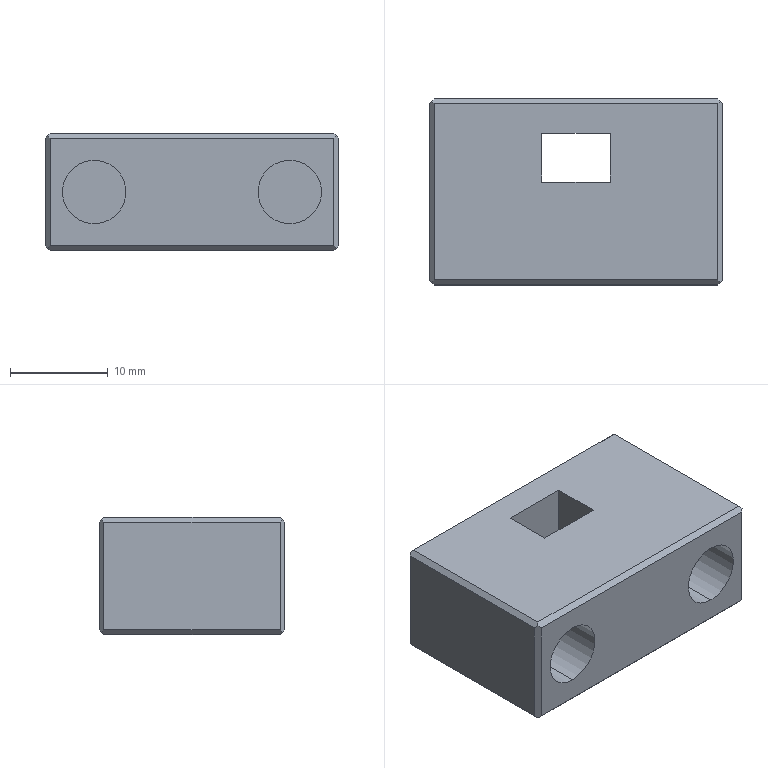Part | SolidWorks | features Chamfer 3, Cut 2, HoleWzd 2, Extrusion 1 | 1 solid | 52 faces | box 30 x 19 x 12 mm | volume 5175 mm3 | plane 24 | cone 16 | cylinder 12 | commonest cylinder face diameters 1.6 x4 3 x4 6.5 x4
STEP:
#1=CARTESIAN_POINT('',(12.5,9.3,-3.6));
#2=VERTEX_POINT('',#1);
#3=CARTESIAN_POINT('',(12.5,9.3,-2.));
#4=VERTEX_POINT('',#3);
#5=CARTESIAN_POINT('',(12.5,9.3,-2.8));
#6=DIRECTION('',(0.,1.,0.));
#7=DIRECTION('',(0.,0.,1.));
#8=AXIS2_PLACEMENT_3D('',#5,#6,#7);
#9=CIRCLE('',#8,0.8);
#10=EDGE_CURVE('',#2,#4,#9,.T.);
#11=ORIENTED_EDGE('',*,*,#10,.F.);
#12=CARTESIAN_POINT('',(12.5,9.5,-3.8));
#13=VERTEX_POINT('',#12);
#14=CARTESIAN_POINT('',(12.5,9.3,-3.6));
#15=DIRECTION('',(0.,0.7071,-0.7071));
#16=VECTOR('',#15,1000.);
#17=LINE('',#14,#16);
#18=EDGE_CURVE('',#2,#13,#17,.T.);
#19=ORIENTED_EDGE('',*,*,#18,.T.);
#20=CARTESIAN_POINT('',(12.5,9.5,-1.8));
#21=VERTEX_POINT('',#20);
#22=CARTESIAN_POINT('',(12.5,9.5,-2.8));
#23=DIRECTION('',(0.,-1.,0.));
#24=DIRECTION('',(0.,0.,1.));
#25=AXIS2_PLACEMENT_3D('',#22,#23,#24);
#26=CIRCLE('',#25,1.);
#27=EDGE_CURVE('',#21,#13,#26,.T.);
#28=ORIENTED_EDGE('',*,*,#27,.F.);
#29=CARTESIAN_POINT('',(12.5,9.3,-2.));
#30=DIRECTION('',(0.,0.7071,0.7071));
#31=VECTOR('',#30,1000.);
#32=LINE('',#29,#31);
#33=EDGE_CURVE('',#4,#21,#32,.T.);
#34=ORIENTED_EDGE('',*,*,#33,.F.);
#35=EDGE_LOOP('',(#11,#19,#28,#34));
#36=FACE_OUTER_BOUND('',#35,.T.);
#37=CARTESIAN_POINT('',(12.5,9.3,-2.8));
#38=DIRECTION('',(0.,1.,0.));
#39=DIRECTION('',(0.,0.,1.));
#40=AXIS2_PLACEMENT_3D('',#37,#38,#39);
#41=CONICAL_SURFACE('',#40,0.8,0.7854);
#42=ADVANCED_FACE('',(#36),#41,.F.);
#43=CARTESIAN_POINT('',(-12.5,9.3,-3.6));
#44=VERTEX_POINT('',#43);
#45=CARTESIAN_POINT('',(-12.5,9.3,-2.));
#46=VERTEX_POINT('',#45);
#47=CARTESIAN_POINT('',(-12.5,9.3,-2.8));
#48=DIRECTION('',(0.,1.,0.));
#49=DIRECTION('',(0.,0.,1.));
#50=AXIS2_PLACEMENT_3D('',#47,#48,#49);
#51=CIRCLE('',#50,0.8);
#52=EDGE_CURVE('',#44,#46,#51,.T.);
#53=ORIENTED_EDGE('',*,*,#52,.F.);
#54=CARTESIAN_POINT('',(-12.5,9.5,-3.8));
#55=VERTEX_POINT('',#54);
#56=CARTESIAN_POINT('',(-12.5,9.3,-3.6));
#57=DIRECTION('',(0.,0.7071,-0.7071));
#58=VECTOR('',#57,1000.);
#59=LINE('',#56,#58);
#60=EDGE_CURVE('',#44,#55,#59,.T.);
#61=ORIENTED_EDGE('',*,*,#60,.T.);
#62=CARTESIAN_POINT('',(-12.5,9.5,-1.8));
#63=VERTEX_POINT('',#62);
#64=CARTESIAN_POINT('',(-12.5,9.5,-2.8));
#65=DIRECTION('',(0.,-1.,0.));
#66=DIRECTION('',(0.,0.,1.));
#67=AXIS2_PLACEMENT_3D('',#64,#65,#66);
#68=CIRCLE('',#67,1.);
#69=EDGE_CURVE('',#63,#55,#68,.T.);
#70=ORIENTED_EDGE('',*,*,#69,.F.);
#71=CARTESIAN_POINT('',(-12.5,9.3,-2.));
#72=DIRECTION('',(0.,0.7071,0.7071));
#73=VECTOR('',#72,1000.);
#74=LINE('',#71,#73);
#75=EDGE_CURVE('',#46,#63,#74,.T.);
#76=ORIENTED_EDGE('',*,*,#75,.F.);
#77=EDGE_LOOP('',(#53,#61,#70,#76));
#78=FACE_OUTER_BOUND('',#77,.T.);
#79=CARTESIAN_POINT('',(-12.5,9.3,-2.8));
#80=DIRECTION('',(0.,1.,0.));
#81=DIRECTION('',(0.,0.,1.));
#82=AXIS2_PLACEMENT_3D('',#79,#80,#81);
#83=CONICAL_SURFACE('',#82,0.8,0.7854);
#84=ADVANCED_FACE('',(#78),#83,.F.);
#85=CARTESIAN_POINT('',(-6.,9.,-4.3));
#86=VERTEX_POINT('',#85);
#87=CARTESIAN_POINT('',(-6.,9.,-1.3));
#88=VERTEX_POINT('',#87);
#89=CARTESIAN_POINT('',(-6.,9.,-2.8));
#90=DIRECTION('',(0.,1.,0.));
#91=DIRECTION('',(0.,0.,1.));
#92=AXIS2_PLACEMENT_3D('',#89,#90,#91);
#93=CIRCLE('',#92,1.5);
#94=EDGE_CURVE('',#86,#88,#93,.T.);
#95=ORIENTED_EDGE('',*,*,#94,.F.);
#96=CARTESIAN_POINT('',(-6.,9.5,-4.8));
#97=VERTEX_POINT('',#96);
#98=CARTESIAN_POINT('',(-6.,9.,-4.3));
#99=DIRECTION('',(0.,0.7071,-0.7071));
#100=VECTOR('',#99,1000.);
#101=LINE('',#98,#100);
#102=EDGE_CURVE('',#86,#97,#101,.T.);
#103=ORIENTED_EDGE('',*,*,#102,.T.);
#104=CARTESIAN_POINT('',(-6.,9.5,-0.8));
#105=VERTEX_POINT('',#104);
#106=CARTESIAN_POINT('',(-6.,9.5,-2.8));
#107=DIRECTION('',(0.,-1.,0.));
#108=DIRECTION('',(0.,0.,1.));
#109=AXIS2_PLACEMENT_3D('',#106,#107,#108);
#110=CIRCLE('',#109,2.);
#111=EDGE_CURVE('',#105,#97,#110,.T.);
#112=ORIENTED_EDGE('',*,*,#111,.F.);
#113=CARTESIAN_POINT('',(-6.,9.,-1.3));
#114=DIRECTION('',(0.,0.7071,0.7071));
#115=VECTOR('',#114,1000.);
#116=LINE('',#113,#115);
#117=EDGE_CURVE('',#88,#105,#116,.T.);
#118=ORIENTED_EDGE('',*,*,#117,.F.);
#119=EDGE_LOOP('',(#95,#103,#112,#118));
#120=FACE_OUTER_BOUND('',#119,.T.);
#121=CARTESIAN_POINT('',(-6.,9.,-2.8));
#122=DIRECTION('',(0.,1.,0.));
#123=DIRECTION('',(0.,0.,1.));
#124=AXIS2_PLACEMENT_3D('',#121,#122,#123);
#125=CONICAL_SURFACE('',#124,1.5,0.7854);
#126=ADVANCED_FACE('',(#120),#125,.F.);
#127=CARTESIAN_POINT('',(6.,9.,-4.3));
#128=VERTEX_POINT('',#127);
#129=CARTESIAN_POINT('',(6.,9.,-1.3));
#130=VERTEX_POINT('',#129);
#131=CARTESIAN_POINT('',(6.,9.,-2.8));
#132=DIRECTION('',(0.,1.,0.));
#133=DIRECTION('',(0.,0.,1.));
#134=AXIS2_PLACEMENT_3D('',#131,#132,#133);
#135=CIRCLE('',#134,1.5);
#136=EDGE_CURVE('',#128,#130,#135,.T.);
#137=ORIENTED_EDGE('',*,*,#136,.F.);
#138=CARTESIAN_POINT('',(6.,9.5,-4.8));
#139=VERTEX_POINT('',#138);
#140=CARTESIAN_POINT('',(6.,9.,-4.3));
#141=DIRECTION('',(0.,0.7071,-0.7071));
#142=VECTOR('',#141,1000.);
#143=LINE('',#140,#142);
#144=EDGE_CURVE('',#128,#139,#143,.T.);
#145=ORIENTED_EDGE('',*,*,#144,.T.);
#146=CARTESIAN_POINT('',(6.,9.5,-0.8));
#147=VERTEX_POINT('',#146);
#148=CARTESIAN_POINT('',(6.,9.5,-2.8));
#149=DIRECTION('',(0.,-1.,0.));
#150=DIRECTION('',(0.,0.,1.));
#151=AXIS2_PLACEMENT_3D('',#148,#149,#150);
#152=CIRCLE('',#151,2.);
#153=EDGE_CURVE('',#147,#139,#152,.T.);
#154=ORIENTED_EDGE('',*,*,#153,.F.);
#155=CARTESIAN_POINT('',(6.,9.,-1.3));
#156=DIRECTION('',(0.,0.7071,0.7071));
#157=VECTOR('',#156,1000.);
#158=LINE('',#155,#157);
#159=EDGE_CURVE('',#130,#147,#158,.T.);
#160=ORIENTED_EDGE('',*,*,#159,.F.);
#161=EDGE_LOOP('',(#137,#145,#154,#160));
#162=FACE_OUTER_BOUND('',#161,.T.);
#163=CARTESIAN_POINT('',(6.,9.,-2.8));
#164=DIRECTION('',(0.,1.,0.));
#165=DIRECTION('',(0.,0.,1.));
#166=AXIS2_PLACEMENT_3D('',#163,#164,#165);
#167=CONICAL_SURFACE('',#166,1.5,0.7854);
#168=ADVANCED_FACE('',(#162),#167,.F.);
#169=CARTESIAN_POINT('',(6.,2.5,-4.3));
#170=VERTEX_POINT('',#169);
#171=CARTESIAN_POINT('',(6.,2.5,-1.3));
#172=VERTEX_POINT('',#171);
#173=CARTESIAN_POINT('',(6.,2.5,-2.8));
#174=DIRECTION('',(0.,1.,0.));
#175=DIRECTION('',(0.,0.,1.));
#176=AXIS2_PLACEMENT_3D('',#173,#174,#175);
#177=CIRCLE('',#176,1.5);
#178=EDGE_CURVE('',#170,#172,#177,.T.);
#179=ORIENTED_EDGE('',*,*,#178,.F.);
#180=CARTESIAN_POINT('',(6.,9.5,-4.3));
#181=DIRECTION('',(0.,1.,0.));
#182=VECTOR('',#181,1000.);
#183=LINE('',#180,#182);
#184=EDGE_CURVE('',#170,#128,#183,.T.);
#185=ORIENTED_EDGE('',*,*,#184,.T.);
#186=ORIENTED_EDGE('',*,*,#136,.T.);
#187=CARTESIAN_POINT('',(6.,9.5,-1.3));
#188=DIRECTION('',(0.,1.,0.));
#189=VECTOR('',#188,1000.);
#190=LINE('',#187,#189);
#191=EDGE_CURVE('',#172,#130,#190,.T.);
#192=ORIENTED_EDGE('',*,*,#191,.F.);
#193=EDGE_LOOP('',(#179,#185,#186,#192));
#194=FACE_OUTER_BOUND('',#193,.T.);
#195=CARTESIAN_POINT('',(6.,9.5,-2.8));
#196=DIRECTION('',(0.,1.,0.));
#197=DIRECTION('',(0.,0.,1.));
#198=AXIS2_PLACEMENT_3D('',#195,#196,#197);
#199=CYLINDRICAL_SURFACE('',#198,1.5);
#200=ADVANCED_FACE('',(#194),#199,.F.);
#201=CARTESIAN_POINT('',(6.,1.599,-2.8));
#202=VERTEX_POINT('',#201);
#203=CARTESIAN_POINT('',(6.,2.5,-1.3));
#204=DIRECTION('',(0.,0.515,0.8572));
#205=VECTOR('',#204,1000.);
#206=LINE('',#203,#205);
#207=EDGE_CURVE('',#202,#172,#206,.T.);
#208=ORIENTED_EDGE('',*,*,#207,.F.);
#209=CARTESIAN_POINT('',(6.,2.5,-4.3));
#210=DIRECTION('',(0.,0.515,-0.8572));
#211=VECTOR('',#210,1000.);
#212=LINE('',#209,#211);
#213=EDGE_CURVE('',#202,#170,#212,.T.);
#214=ORIENTED_EDGE('',*,*,#213,.T.);
#215=ORIENTED_EDGE('',*,*,#178,.T.);
#216=EDGE_LOOP('',(#208,#214,#215));
#217=FACE_OUTER_BOUND('',#216,.T.);
#218=CARTESIAN_POINT('',(6.,2.5,-2.8));
#219=DIRECTION('',(0.,1.,0.));
#220=DIRECTION('',(0.,0.,1.));
#221=AXIS2_PLACEMENT_3D('',#218,#219,#220);
#222=CONICAL_SURFACE('',#221,1.5,1.03);
#223=ADVANCED_FACE('',(#217),#222,.F.);
#224=CARTESIAN_POINT('',(-6.,2.5,-4.3));
#225=VERTEX_POINT('',#224);
#226=CARTESIAN_POINT('',(-6.,2.5,-1.3));
#227=VERTEX_POINT('',#226);
#228=CARTESIAN_POINT('',(-6.,2.5,-2.8));
#229=DIRECTION('',(0.,1.,0.));
#230=DIRECTION('',(0.,0.,1.));
#231=AXIS2_PLACEMENT_3D('',#228,#229,#230);
#232=CIRCLE('',#231,1.5);
#233=EDGE_CURVE('',#225,#227,#232,.T.);
#234=ORIENTED_EDGE('',*,*,#233,.F.);
#235=CARTESIAN_POINT('',(-6.,9.5,-4.3));
#236=DIRECTION('',(0.,1.,0.));
#237=VECTOR('',#236,1000.);
#238=LINE('',#235,#237);
#239=EDGE_CURVE('',#225,#86,#238,.T.);
#240=ORIENTED_EDGE('',*,*,#239,.T.);
#241=ORIENTED_EDGE('',*,*,#94,.T.);
#242=CARTESIAN_POINT('',(-6.,9.5,-1.3));
#243=DIRECTION('',(0.,1.,0.));
#244=VECTOR('',#243,1000.);
#245=LINE('',#242,#244);
#246=EDGE_CURVE('',#227,#88,#245,.T.);
#247=ORIENTED_EDGE('',*,*,#246,.F.);
#248=EDGE_LOOP('',(#234,#240,#241,#247));
#249=FACE_OUTER_BOUND('',#248,.T.);
#250=CARTESIAN_POINT('',(-6.,9.5,-2.8));
#251=DIRECTION('',(0.,1.,0.));
#252=DIRECTION('',(0.,0.,1.));
#253=AXIS2_PLACEMENT_3D('',#250,#251,#252);
#254=CYLINDRICAL_SURFACE('',#253,1.5);
#255=ADVANCED_FACE('',(#249),#254,.F.);
#256=CARTESIAN_POINT('',(-6.,1.599,-2.8));
#257=VERTEX_POINT('',#256);
#258=CARTESIAN_POINT('',(-6.,2.5,-1.3));
#259=DIRECTION('',(0.,0.515,0.8572));
#260=VECTOR('',#259,1000.);
#261=LINE('',#258,#260);
#262=EDGE_CURVE('',#257,#227,#261,.T.);
#263=ORIENTED_EDGE('',*,*,#262,.F.);
#264=CARTESIAN_POINT('',(-6.,2.5,-4.3));
#265=DIRECTION('',(0.,0.515,-0.8572));
#266=VECTOR('',#265,1000.);
#267=LINE('',#264,#266);
#268=EDGE_CURVE('',#257,#225,#267,.T.);
#269=ORIENTED_EDGE('',*,*,#268,.T.);
#270=ORIENTED_EDGE('',*,*,#233,.T.);
#271=EDGE_LOOP('',(#263,#269,#270));
#272=FACE_OUTER_BOUND('',#271,.T.);
#273=CARTESIAN_POINT('',(-6.,2.5,-2.8));
#274=DIRECTION('',(0.,1.,0.));
#275=DIRECTION('',(0.,0.,1.));
#276=AXIS2_PLACEMENT_3D('',#273,#274,#275);
#277=CONICAL_SURFACE('',#276,1.5,1.03);
#278=ADVANCED_FACE('',(#272),#277,.F.);
#279=CARTESIAN_POINT('',(-12.5,4.3,-3.6));
#280=VERTEX_POINT('',#279);
#281=CARTESIAN_POINT('',(-12.5,4.3,-2.));
#282=VERTEX_POINT('',#281);
#283=CARTESIAN_POINT('',(-12.5,4.3,-2.8));
#284=DIRECTION('',(0.,1.,0.));
#285=DIRECTION('',(0.,0.,1.));
#286=AXIS2_PLACEMENT_3D('',#283,#284,#285);
#287=CIRCLE('',#286,0.8);
#288=EDGE_CURVE('',#280,#282,#287,.T.);
#289=ORIENTED_EDGE('',*,*,#288,.F.);
#290=CARTESIAN_POINT('',(-12.5,9.5,-3.6));
#291=DIRECTION('',(0.,1.,0.));
#292=VECTOR('',#291,1000.);
#293=LINE('',#290,#292);
#294=EDGE_CURVE('',#280,#44,#293,.T.);
#295=ORIENTED_EDGE('',*,*,#294,.T.);
#296=ORIENTED_EDGE('',*,*,#52,.T.);
#297=CARTESIAN_POINT('',(-12.5,9.5,-2.));
#298=DIRECTION('',(0.,1.,0.));
#299=VECTOR('',#298,1000.);
#300=LINE('',#297,#299);
#301=EDGE_CURVE('',#282,#46,#300,.T.);
#302=ORIENTED_EDGE('',*,*,#301,.F.);
#303=EDGE_LOOP('',(#289,#295,#296,#302));
#304=FACE_OUTER_BOUND('',#303,.T.);
#305=CARTESIAN_POINT('',(-12.5,9.5,-2.8));
#306=DIRECTION('',(0.,1.,0.));
#307=DIRECTION('',(0.,0.,1.));
#308=AXIS2_PLACEMENT_3D('',#305,#306,#307);
#309=CYLINDRICAL_SURFACE('',#308,0.8);
#310=ADVANCED_FACE('',(#304),#309,.F.);
#311=CARTESIAN_POINT('',(-12.5,3.819,-2.8));
#312=VERTEX_POINT('',#311);
#313=CARTESIAN_POINT('',(-12.5,4.3,-2.));
#314=DIRECTION('',(0.,0.515,0.8572));
#315=VECTOR('',#314,1000.);
#316=LINE('',#313,#315);
#317=EDGE_CURVE('',#312,#282,#316,.T.);
#318=ORIENTED_EDGE('',*,*,#317,.F.);
#319=CARTESIAN_POINT('',(-12.5,4.3,-3.6));
#320=DIRECTION('',(0.,0.515,-0.8572));
#321=VECTOR('',#320,1000.);
#322=LINE('',#319,#321);
#323=EDGE_CURVE('',#312,#280,#322,.T.);
#324=ORIENTED_EDGE('',*,*,#323,.T.);
#325=ORIENTED_EDGE('',*,*,#288,.T.);
#326=EDGE_LOOP('',(#318,#324,#325));
#327=FACE_OUTER_BOUND('',#326,.T.);
#328=CARTESIAN_POINT('',(-12.5,4.3,-2.8));
#329=DIRECTION('',(0.,1.,0.));
#330=DIRECTION('',(0.,0.,1.));
#331=AXIS2_PLACEMENT_3D('',#328,#329,#330);
#332=CONICAL_SURFACE('',#331,0.8,1.03);
#333=ADVANCED_FACE('',(#327),#332,.F.);
#334=CARTESIAN_POINT('',(12.5,4.3,-3.6));
#335=VERTEX_POINT('',#334);
#336=CARTESIAN_POINT('',(12.5,4.3,-2.));
#337=VERTEX_POINT('',#336);
#338=CARTESIAN_POINT('',(12.5,4.3,-2.8));
#339=DIRECTION('',(0.,1.,0.));
#340=DIRECTION('',(0.,0.,1.));
#341=AXIS2_PLACEMENT_3D('',#338,#339,#340);
#342=CIRCLE('',#341,0.8);
#343=EDGE_CURVE('',#335,#337,#342,.T.);
#344=ORIENTED_EDGE('',*,*,#343,.F.);
#345=CARTESIAN_POINT('',(12.5,9.5,-3.6));
#346=DIRECTION('',(0.,1.,0.));
#347=VECTOR('',#346,1000.);
#348=LINE('',#345,#347);
#349=EDGE_CURVE('',#335,#2,#348,.T.);
#350=ORIENTED_EDGE('',*,*,#349,.T.);
#351=ORIENTED_EDGE('',*,*,#10,.T.);
#352=CARTESIAN_POINT('',(12.5,9.5,-2.));
#353=DIRECTION('',(0.,1.,0.));
#354=VECTOR('',#353,1000.);
#355=LINE('',#352,#354);
#356=EDGE_CURVE('',#337,#4,#355,.T.);
#357=ORIENTED_EDGE('',*,*,#356,.F.);
#358=EDGE_LOOP('',(#344,#350,#351,#357));
#359=FACE_OUTER_BOUND('',#358,.T.);
#360=CARTESIAN_POINT('',(12.5,9.5,-2.8));
#361=DIRECTION('',(0.,1.,0.));
#362=DIRECTION('',(0.,0.,1.));
#363=AXIS2_PLACEMENT_3D('',#360,#361,#362);
#364=CYLINDRICAL_SURFACE('',#363,0.8);
#365=ADVANCED_FACE('',(#359),#364,.F.);
#366=CARTESIAN_POINT('',(12.5,3.819,-2.8));
#367=VERTEX_POINT('',#366);
#368=CARTESIAN_POINT('',(12.5,4.3,-2.));
#369=DIRECTION('',(0.,0.515,0.8572));
#370=VECTOR('',#369,1000.);
#371=LINE('',#368,#370);
#372=EDGE_CURVE('',#367,#337,#371,.T.);
#373=ORIENTED_EDGE('',*,*,#372,.F.);
#374=CARTESIAN_POINT('',(12.5,4.3,-3.6));
#375=DIRECTION('',(0.,0.515,-0.8572));
#376=VECTOR('',#375,1000.);
#377=LINE('',#374,#376);
#378=EDGE_CURVE('',#367,#335,#377,.T.);
#379=ORIENTED_EDGE('',*,*,#378,.T.);
#380=ORIENTED_EDGE('',*,*,#343,.T.);
#381=EDGE_LOOP('',(#373,#379,#380));
#382=FACE_OUTER_BOUND('',#381,.T.);
#383=CARTESIAN_POINT('',(12.5,4.3,-2.8));
#384=DIRECTION('',(0.,1.,0.));
#385=DIRECTION('',(0.,0.,1.));
#386=AXIS2_PLACEMENT_3D('',#383,#384,#385);
#387=CONICAL_SURFACE('',#386,0.8,1.03);
#388=ADVANCED_FACE('',(#382),#387,.F.);
#389=CARTESIAN_POINT('',(-10.,2.5,-9.25));
#390=VERTEX_POINT('',#389);
#391=CARTESIAN_POINT('',(-10.,2.5,-2.75));
#392=VERTEX_POINT('',#391);
#393=CARTESIAN_POINT('',(-10.,2.5,-6.));
#394=DIRECTION('',(0.,1.,0.));
#395=DIRECTION('',(0.,0.,-1.));
#396=AXIS2_PLACEMENT_3D('',#393,#394,#395);
#397=CIRCLE('',#396,3.25);
#398=EDGE_CURVE('',#390,#392,#397,.T.);
#399=ORIENTED_EDGE('',*,*,#398,.T.);
#400=CARTESIAN_POINT('',(-10.,-9.5,-2.75));
#401=VERTEX_POINT('',#400);
#402=CARTESIAN_POINT('',(-10.,11.692,-2.75));
#403=DIRECTION('',(0.,-1.,0.));
#404=VECTOR('',#403,1000.);
#405=LINE('',#402,#404);
#406=EDGE_CURVE('',#392,#401,#405,.T.);
#407=ORIENTED_EDGE('',*,*,#406,.T.);
#408=CARTESIAN_POINT('',(-10.,-9.5,-9.25));
#409=VERTEX_POINT('',#408);
#410=CARTESIAN_POINT('',(-10.,-9.5,-6.));
#411=DIRECTION('',(0.,-1.,0.));
#412=DIRECTION('',(0.,0.,-1.));
#413=AXIS2_PLACEMENT_3D('',#410,#411,#412);
#414=CIRCLE('',#413,3.25);
#415=EDGE_CURVE('',#401,#409,#414,.T.);
#416=ORIENTED_EDGE('',*,*,#415,.T.);
#417=CARTESIAN_POINT('',(-10.,11.692,-9.25));
#418=DIRECTION('',(0.,-1.,0.));
#419=VECTOR('',#418,1000.);
#420=LINE('',#417,#419);
#421=EDGE_CURVE('',#390,#409,#420,.T.);
#422=ORIENTED_EDGE('',*,*,#421,.F.);
#423=EDGE_LOOP('',(#399,#407,#416,#422));
#424=FACE_OUTER_BOUND('',#423,.T.);
#425=CARTESIAN_POINT('',(-10.,11.692,-6.));
#426=DIRECTION('',(0.,-1.,0.));
#427=DIRECTION('',(0.,0.,-1.));
#428=AXIS2_PLACEMENT_3D('',#425,#426,#427);
#429=CYLINDRICAL_SURFACE('',#428,3.25);
#430=ADVANCED_FACE('',(#424),#429,.F.);
#431=CARTESIAN_POINT('',(10.,2.5,-2.75));
#432=VERTEX_POINT('',#431);
#433=CARTESIAN_POINT('',(10.,2.5,-9.25));
#434=VERTEX_POINT('',#433);
#435=CARTESIAN_POINT('',(10.,2.5,-6.));
#436=DIRECTION('',(0.,-1.,0.));
#437=DIRECTION('',(0.,0.,-1.));
#438=AXIS2_PLACEMENT_3D('',#435,#436,#437);
#439=CIRCLE('',#438,3.25);
#440=EDGE_CURVE('',#432,#434,#439,.T.);
#441=ORIENTED_EDGE('',*,*,#440,.F.);
#442=CARTESIAN_POINT('',(10.,-9.5,-2.75));
#443=VERTEX_POINT('',#442);
#444=CARTESIAN_POINT('',(10.,11.692,-2.75));
#445=DIRECTION('',(0.,-1.,0.));
#446=VECTOR('',#445,1000.);
#447=LINE('',#444,#446);
#448=EDGE_CURVE('',#432,#443,#447,.T.);
#449=ORIENTED_EDGE('',*,*,#448,.T.);
#450=CARTESIAN_POINT('',(10.,-9.5,-9.25));
#451=VERTEX_POINT('',#450);
#452=CARTESIAN_POINT('',(10.,-9.5,-6.));
#453=DIRECTION('',(0.,-1.,0.));
#454=DIRECTION('',(0.,0.,-1.));
#455=AXIS2_PLACEMENT_3D('',#452,#453,#454);
#456=CIRCLE('',#455,3.25);
#457=EDGE_CURVE('',#443,#451,#456,.T.);
#458=ORIENTED_EDGE('',*,*,#457,.T.);
#459=CARTESIAN_POINT('',(10.,11.692,-9.25));
#460=DIRECTION('',(0.,-1.,0.));
#461=VECTOR('',#460,1000.);
#462=LINE('',#459,#461);
#463=EDGE_CURVE('',#434,#451,#462,.T.);
#464=ORIENTED_EDGE('',*,*,#463,.F.);
#465=EDGE_LOOP('',(#441,#449,#458,#464));
#466=FACE_OUTER_BOUND('',#465,.T.);
#467=CARTESIAN_POINT('',(10.,11.692,-6.));
#468=DIRECTION('',(0.,-1.,0.));
#469=DIRECTION('',(0.,0.,-1.));
#470=AXIS2_PLACEMENT_3D('',#467,#468,#469);
#471=CYLINDRICAL_SURFACE('',#470,3.25);
#472=ADVANCED_FACE('',(#466),#471,.F.);
#473=CARTESIAN_POINT('',(14.5,-9.,0.));
#474=VERTEX_POINT('',#473);
#475=CARTESIAN_POINT('',(14.5,9.,0.));
#476=VERTEX_POINT('',#475);
#477=CARTESIAN_POINT('',(14.5,0.,0.));
#478=DIRECTION('',(0.,1.,0.));
#479=VECTOR('',#478,1000.);
#480=LINE('',#477,#479);
#481=EDGE_CURVE('',#474,#476,#480,.T.);
#482=ORIENTED_EDGE('',*,*,#481,.T.);
#483=CARTESIAN_POINT('',(-14.5,9.,0.));
#484=VERTEX_POINT('',#483);
#485=CARTESIAN_POINT('',(0.,9.,0.));
#486=DIRECTION('',(-1.,0.,0.));
#487=VECTOR('',#486,1000.);
#488=LINE('',#485,#487);
#489=EDGE_CURVE('',#476,#484,#488,.T.);
#490=ORIENTED_EDGE('',*,*,#489,.T.);
#491=CARTESIAN_POINT('',(-14.5,-9.,0.));
#492=VERTEX_POINT('',#491);
#493=CARTESIAN_POINT('',(-14.5,0.,0.));
#494=DIRECTION('',(0.,-1.,0.));
#495=VECTOR('',#494,1000.);
#496=LINE('',#493,#495);
#497=EDGE_CURVE('',#484,#492,#496,.T.);
#498=ORIENTED_EDGE('',*,*,#497,.T.);
#499=CARTESIAN_POINT('',(0.,-9.,0.));
#500=DIRECTION('',(1.,0.,0.));
#501=VECTOR('',#500,1000.);
#502=LINE('',#499,#501);
#503=EDGE_CURVE('',#492,#474,#502,.T.);
#504=ORIENTED_EDGE('',*,*,#503,.T.);
#505=EDGE_LOOP('',(#482,#490,#498,#504));
#506=FACE_OUTER_BOUND('',#505,.T.);
#507=CARTESIAN_POINT('',(3.5,1.,0.));
#508=VERTEX_POINT('',#507);
#509=CARTESIAN_POINT('',(-3.5,1.,0.));
#510=VERTEX_POINT('',#509);
#511=CARTESIAN_POINT('',(20.42,1.,0.));
#512=DIRECTION('',(-1.,0.,0.));
#513=VECTOR('',#512,1000.);
#514=LINE('',#511,#513);
#515=EDGE_CURVE('',#508,#510,#514,.T.);
#516=ORIENTED_EDGE('',*,*,#515,.T.);
#517=CARTESIAN_POINT('',(-3.5,6.,0.));
#518=VERTEX_POINT('',#517);
#519=CARTESIAN_POINT('',(-3.5,6.,0.));
#520=DIRECTION('',(0.,-1.,0.));
#521=VECTOR('',#520,1000.);
#522=LINE('',#519,#521);
#523=EDGE_CURVE('',#518,#510,#522,.T.);
#524=ORIENTED_EDGE('',*,*,#523,.F.);
#525=CARTESIAN_POINT('',(3.5,6.,0.));
#526=VERTEX_POINT('',#525);
#527=CARTESIAN_POINT('',(20.42,6.,0.));
#528=DIRECTION('',(-1.,0.,0.));
#529=VECTOR('',#528,1000.);
#530=LINE('',#527,#529);
#531=EDGE_CURVE('',#526,#518,#530,.T.);
#532=ORIENTED_EDGE('',*,*,#531,.F.);
#533=CARTESIAN_POINT('',(3.5,6.,0.));
#534=DIRECTION('',(0.,-1.,0.));
#535=VECTOR('',#534,1000.);
#536=LINE('',#533,#535);
#537=EDGE_CURVE('',#526,#508,#536,.T.);
#538=ORIENTED_EDGE('',*,*,#537,.T.);
#539=EDGE_LOOP('',(#516,#524,#532,#538));
#540=FACE_BOUND('',#539,.T.);
#541=CARTESIAN_POINT('',(0.,0.,0.));
#542=DIRECTION('',(0.,0.,1.));
#543=DIRECTION('',(1.,0.,0.));
#544=AXIS2_PLACEMENT_3D('',#541,#542,#543);
#545=PLANE('',#544);
#546=ADVANCED_FACE('',(#506,#540),#545,.T.);
#547=CARTESIAN_POINT('',(-14.5,9.,-12.));
#548=VERTEX_POINT('',#547);
#549=CARTESIAN_POINT('',(14.5,9.,-12.));
#550=VERTEX_POINT('',#549);
#551=CARTESIAN_POINT('',(14.5,9.,-12.));
#552=DIRECTION('',(1.,0.,0.));
#553=VECTOR('',#552,1000.);
#554=LINE('',#551,#553);
#555=EDGE_CURVE('',#548,#550,#554,.T.);
#556=ORIENTED_EDGE('',*,*,#555,.T.);
#557=CARTESIAN_POINT('',(14.5,-9.,-12.));
#558=VERTEX_POINT('',#557);
#559=CARTESIAN_POINT('',(14.5,-9.,-12.));
#560=DIRECTION('',(0.,-1.,0.));
#561=VECTOR('',#560,1000.);
#562=LINE('',#559,#561);
#563=EDGE_CURVE('',#550,#558,#562,.T.);
#564=ORIENTED_EDGE('',*,*,#563,.T.);
#565=CARTESIAN_POINT('',(-14.5,-9.,-12.));
#566=VERTEX_POINT('',#565);
#567=CARTESIAN_POINT('',(-14.5,-9.,-12.));
#568=DIRECTION('',(-1.,0.,0.));
#569=VECTOR('',#568,1000.);
#570=LINE('',#567,#569);
#571=EDGE_CURVE('',#558,#566,#570,.T.);
#572=ORIENTED_EDGE('',*,*,#571,.T.);
#573=CARTESIAN_POINT('',(-14.5,9.,-12.));
#574=DIRECTION('',(0.,1.,0.));
#575=VECTOR('',#574,1000.);
#576=LINE('',#573,#575);
#577=EDGE_CURVE('',#566,#548,#576,.T.);
#578=ORIENTED_EDGE('',*,*,#577,.T.);
#579=EDGE_LOOP('',(#556,#564,#572,#578));
#580=FACE_OUTER_BOUND('',#579,.T.);
#581=CARTESIAN_POINT('',(-3.5,-5.928,-12.));
#582=VERTEX_POINT('',#581);
#583=CARTESIAN_POINT('',(-3.5,6.,-12.));
#584=VERTEX_POINT('',#583);
#585=CARTESIAN_POINT('',(-3.5,-5.928,-12.));
#586=DIRECTION('',(0.,1.,0.));
#587=VECTOR('',#586,1000.);
#588=LINE('',#585,#587);
#589=EDGE_CURVE('',#582,#584,#588,.T.);
#590=ORIENTED_EDGE('',*,*,#589,.F.);
#591=CARTESIAN_POINT('',(3.5,-5.928,-12.));
#592=VERTEX_POINT('',#591);
#593=CARTESIAN_POINT('',(20.42,-5.928,-12.));
#594=DIRECTION('',(-1.,0.,0.));
#595=VECTOR('',#594,1000.);
#596=LINE('',#593,#595);
#597=EDGE_CURVE('',#592,#582,#596,.T.);
#598=ORIENTED_EDGE('',*,*,#597,.F.);
#599=CARTESIAN_POINT('',(3.5,6.,-12.));
#600=VERTEX_POINT('',#599);
#601=CARTESIAN_POINT('',(3.5,-5.928,-12.));
#602=DIRECTION('',(0.,1.,0.));
#603=VECTOR('',#602,1000.);
#604=LINE('',#601,#603);
#605=EDGE_CURVE('',#592,#600,#604,.T.);
#606=ORIENTED_EDGE('',*,*,#605,.T.);
#607=CARTESIAN_POINT('',(20.42,6.,-12.));
#608=DIRECTION('',(-1.,0.,0.));
#609=VECTOR('',#608,1000.);
#610=LINE('',#607,#609);
#611=EDGE_CURVE('',#600,#584,#610,.T.);
#612=ORIENTED_EDGE('',*,*,#611,.T.);
#613=EDGE_LOOP('',(#590,#598,#606,#612));
#614=FACE_BOUND('',#613,.T.);
#615=CARTESIAN_POINT('',(0.,0.,-12.));
#616=DIRECTION('',(0.,0.,1.));
#617=DIRECTION('',(1.,0.,0.));
#618=AXIS2_PLACEMENT_3D('',#615,#616,#617);
#619=PLANE('',#618);
#620=ADVANCED_FACE('',(#580,#614),#619,.F.);
#621=CARTESIAN_POINT('',(-14.5,9.5,-11.5));
#622=VERTEX_POINT('',#621);
#623=CARTESIAN_POINT('',(-14.5,9.5,-0.5));
#624=VERTEX_POINT('',#623);
#625=CARTESIAN_POINT('',(-14.5,9.5,-47.511));
#626=DIRECTION('',(0.,0.,1.));
#627=VECTOR('',#626,1000.);
#628=LINE('',#625,#627);
#629=EDGE_CURVE('',#622,#624,#628,.T.);
#630=ORIENTED_EDGE('',*,*,#629,.F.);
#631=CARTESIAN_POINT('',(-14.75,9.25,-11.75));
#632=VERTEX_POINT('',#631);
#633=CARTESIAN_POINT('',(-26.504,-2.504,-23.504));
#634=DIRECTION('',(-0.5774,-0.5774,-0.5774));
#635=VECTOR('',#634,1000.);
#636=LINE('',#633,#635);
#637=EDGE_CURVE('',#622,#632,#636,.T.);
#638=ORIENTED_EDGE('',*,*,#637,.T.);
#639=CARTESIAN_POINT('',(-15.,9.,-11.5));
#640=VERTEX_POINT('',#639);
#641=CARTESIAN_POINT('',(-2.663,21.337,-23.837));
#642=DIRECTION('',(-0.5774,-0.5774,0.5774));
#643=VECTOR('',#642,1000.);
#644=LINE('',#641,#643);
#645=EDGE_CURVE('',#632,#640,#644,.T.);
#646=ORIENTED_EDGE('',*,*,#645,.T.);
#647=CARTESIAN_POINT('',(-15.,9.,-0.5));
#648=VERTEX_POINT('',#647);
#649=CARTESIAN_POINT('',(-15.,9.,-47.511));
#650=DIRECTION('',(0.,0.,1.));
#651=VECTOR('',#650,1000.);
#652=LINE('',#649,#651);
#653=EDGE_CURVE('',#640,#648,#652,.T.);
#654=ORIENTED_EDGE('',*,*,#653,.T.);
#655=CARTESIAN_POINT('',(-14.75,9.25,-0.25));
#656=VERTEX_POINT('',#655);
#657=CARTESIAN_POINT('',(-30.337,-6.337,-15.837));
#658=DIRECTION('',(0.5774,0.5774,0.5774));
#659=VECTOR('',#658,1000.);
#660=LINE('',#657,#659);
#661=EDGE_CURVE('',#648,#656,#660,.T.);
#662=ORIENTED_EDGE('',*,*,#661,.T.);
#663=CARTESIAN_POINT('',(1.17,25.17,-16.17));
#664=DIRECTION('',(0.5774,0.5774,-0.5774));
#665=VECTOR('',#664,1000.);
#666=LINE('',#663,#665);
#667=EDGE_CURVE('',#656,#624,#666,.T.);
#668=ORIENTED_EDGE('',*,*,#667,.T.);
#669=EDGE_LOOP('',(#630,#638,#646,#654,#662,#668));
#670=FACE_OUTER_BOUND('',#669,.T.);
#671=CARTESIAN_POINT('',(-14.5,9.5,-47.511));
#672=DIRECTION('',(-0.7071,0.7071,0.));
#673=DIRECTION('',(-0.7071,-0.7071,0.));
#674=AXIS2_PLACEMENT_3D('',#671,#672,#673);
#675=PLANE('',#674);
#676=ADVANCED_FACE('',(#670),#675,.T.);
#677=ORIENTED_EDGE('',*,*,#69,.T.);
#678=CARTESIAN_POINT('',(-12.5,9.5,-2.8));
#679=DIRECTION('',(0.,-1.,0.));
#680=DIRECTION('',(0.,0.,1.));
#681=AXIS2_PLACEMENT_3D('',#678,#679,#680);
#682=CIRCLE('',#681,1.);
#683=EDGE_CURVE('',#55,#63,#682,.T.);
#684=ORIENTED_EDGE('',*,*,#683,.T.);
#685=EDGE_LOOP('',(#677,#684));
#686=FACE_BOUND('',#685,.T.);
#687=ORIENTED_EDGE('',*,*,#27,.T.);
#688=CARTESIAN_POINT('',(12.5,9.5,-2.8));
#689=DIRECTION('',(0.,-1.,0.));
#690=DIRECTION('',(0.,0.,1.));
#691=AXIS2_PLACEMENT_3D('',#688,#689,#690);
#692=CIRCLE('',#691,1.);
#693=EDGE_CURVE('',#13,#21,#692,.T.);
#694=ORIENTED_EDGE('',*,*,#693,.T.);
#695=EDGE_LOOP('',(#687,#694));
#696=FACE_BOUND('',#695,.T.);
#697=ORIENTED_EDGE('',*,*,#153,.T.);
#698=CARTESIAN_POINT('',(6.,9.5,-2.8));
#699=DIRECTION('',(0.,-1.,0.));
#700=DIRECTION('',(0.,0.,1.));
#701=AXIS2_PLACEMENT_3D('',#698,#699,#700);
#702=CIRCLE('',#701,2.);
#703=EDGE_CURVE('',#139,#147,#702,.T.);
#704=ORIENTED_EDGE('',*,*,#703,.T.);
#705=EDGE_LOOP('',(#697,#704));
#706=FACE_BOUND('',#705,.T.);
#707=ORIENTED_EDGE('',*,*,#111,.T.);
#708=CARTESIAN_POINT('',(-6.,9.5,-2.8));
#709=DIRECTION('',(0.,-1.,0.));
#710=DIRECTION('',(0.,0.,1.));
#711=AXIS2_PLACEMENT_3D('',#708,#709,#710);
#712=CIRCLE('',#711,2.);
#713=EDGE_CURVE('',#97,#105,#712,.T.);
#714=ORIENTED_EDGE('',*,*,#713,.T.);
#715=EDGE_LOOP('',(#707,#714));
#716=FACE_BOUND('',#715,.T.);
#717=CARTESIAN_POINT('',(14.5,9.5,-11.5));
#718=VERTEX_POINT('',#717);
#719=CARTESIAN_POINT('',(14.5,9.5,-0.5));
#720=VERTEX_POINT('',#719);
#721=CARTESIAN_POINT('',(14.5,9.5,-47.511));
#722=DIRECTION('',(0.,0.,1.));
#723=VECTOR('',#722,1000.);
#724=LINE('',#721,#723);
#725=EDGE_CURVE('',#718,#720,#724,.T.);
#726=ORIENTED_EDGE('',*,*,#725,.F.);
#727=CARTESIAN_POINT('',(-14.5,9.5,-11.5));
#728=DIRECTION('',(-1.,0.,0.));
#729=VECTOR('',#728,1000.);
#730=LINE('',#727,#729);
#731=EDGE_CURVE('',#718,#622,#730,.T.);
#732=ORIENTED_EDGE('',*,*,#731,.T.);
#733=ORIENTED_EDGE('',*,*,#629,.T.);
#734=CARTESIAN_POINT('',(14.5,9.5,-0.5));
#735=DIRECTION('',(1.,0.,0.));
#736=VECTOR('',#735,1000.);
#737=LINE('',#734,#736);
#738=EDGE_CURVE('',#624,#720,#737,.T.);
#739=ORIENTED_EDGE('',*,*,#738,.T.);
#740=EDGE_LOOP('',(#726,#732,#733,#739));
#741=FACE_OUTER_BOUND('',#740,.T.);
#742=CARTESIAN_POINT('',(14.5,9.5,-47.511));
#743=DIRECTION('',(0.,1.,0.));
#744=DIRECTION('',(0.,0.,1.));
#745=AXIS2_PLACEMENT_3D('',#742,#743,#744);
#746=PLANE('',#745);
#747=ADVANCED_FACE('',(#686,#696,#706,#716,#741),#746,.T.);
#748=CARTESIAN_POINT('',(15.,9.,-11.5));
#749=VERTEX_POINT('',#748);
#750=CARTESIAN_POINT('',(15.,9.,-0.5));
#751=VERTEX_POINT('',#750);
#752=CARTESIAN_POINT('',(15.,9.,-47.511));
#753=DIRECTION('',(0.,0.,1.));
#754=VECTOR('',#753,1000.);
#755=LINE('',#752,#754);
#756=EDGE_CURVE('',#749,#751,#755,.T.);
#757=ORIENTED_EDGE('',*,*,#756,.F.);
#758=CARTESIAN_POINT('',(14.75,9.25,-11.75));
#759=VERTEX_POINT('',#758);
#760=CARTESIAN_POINT('',(2.996,21.004,-23.504));
#761=DIRECTION('',(-0.5774,0.5774,-0.5774));
#762=VECTOR('',#761,1000.);
#763=LINE('',#760,#762);
#764=EDGE_CURVE('',#749,#759,#763,.T.);
#765=ORIENTED_EDGE('',*,*,#764,.T.);
#766=CARTESIAN_POINT('',(26.837,-2.837,-23.837));
#767=DIRECTION('',(-0.5774,0.5774,0.5774));
#768=VECTOR('',#767,1000.);
#769=LINE('',#766,#768);
#770=EDGE_CURVE('',#759,#718,#769,.T.);
#771=ORIENTED_EDGE('',*,*,#770,.T.);
#772=ORIENTED_EDGE('',*,*,#725,.T.);
#773=CARTESIAN_POINT('',(14.75,9.25,-0.25));
#774=VERTEX_POINT('',#773);
#775=CARTESIAN_POINT('',(-0.8369,24.837,-15.837));
#776=DIRECTION('',(0.5774,-0.5774,0.5774));
#777=VECTOR('',#776,1000.);
#778=LINE('',#775,#777);
#779=EDGE_CURVE('',#720,#774,#778,.T.);
#780=ORIENTED_EDGE('',*,*,#779,.T.);
#781=CARTESIAN_POINT('',(30.67,-6.67,-16.17));
#782=DIRECTION('',(0.5774,-0.5774,-0.5774));
#783=VECTOR('',#782,1000.);
#784=LINE('',#781,#783);
#785=EDGE_CURVE('',#774,#751,#784,.T.);
#786=ORIENTED_EDGE('',*,*,#785,.T.);
#787=EDGE_LOOP('',(#757,#765,#771,#772,#780,#786));
#788=FACE_OUTER_BOUND('',#787,.T.);
#789=CARTESIAN_POINT('',(15.,9.,-47.511));
#790=DIRECTION('',(0.7071,0.7071,0.));
#791=DIRECTION('',(-0.7071,0.7071,0.));
#792=AXIS2_PLACEMENT_3D('',#789,#790,#791);
#793=PLANE('',#792);
#794=ADVANCED_FACE('',(#788),#793,.T.);
#795=CARTESIAN_POINT('',(15.,-9.,-11.5));
#796=VERTEX_POINT('',#795);
#797=CARTESIAN_POINT('',(15.,-9.,-0.5));
#798=VERTEX_POINT('',#797);
#799=CARTESIAN_POINT('',(15.,-9.,-47.511));
#800=DIRECTION('',(0.,0.,1.));
#801=VECTOR('',#800,1000.);
#802=LINE('',#799,#801);
#803=EDGE_CURVE('',#796,#798,#802,.T.);
#804=ORIENTED_EDGE('',*,*,#803,.F.);
#805=CARTESIAN_POINT('',(15.,9.,-11.5));
#806=DIRECTION('',(0.,1.,0.));
#807=VECTOR('',#806,1000.);
#808=LINE('',#805,#807);
#809=EDGE_CURVE('',#796,#749,#808,.T.);
#810=ORIENTED_EDGE('',*,*,#809,.T.);
#811=ORIENTED_EDGE('',*,*,#756,.T.);
#812=CARTESIAN_POINT('',(15.,-9.,-0.5));
#813=DIRECTION('',(0.,-1.,0.));
#814=VECTOR('',#813,1000.);
#815=LINE('',#812,#814);
#816=EDGE_CURVE('',#751,#798,#815,.T.);
#817=ORIENTED_EDGE('',*,*,#816,.T.);
#818=EDGE_LOOP('',(#804,#810,#811,#817));
#819=FACE_OUTER_BOUND('',#818,.T.);
#820=CARTESIAN_POINT('',(15.,-9.,-47.511));
#821=DIRECTION('',(1.,0.,0.));
#822=DIRECTION('',(0.,0.,-1.));
#823=AXIS2_PLACEMENT_3D('',#820,#821,#822);
#824=PLANE('',#823);
#825=ADVANCED_FACE('',(#819),#824,.T.);
#826=CARTESIAN_POINT('',(14.5,-9.5,-11.5));
#827=VERTEX_POINT('',#826);
#828=CARTESIAN_POINT('',(14.75,-9.25,-11.75));
#829=VERTEX_POINT('',#828);
#830=CARTESIAN_POINT('',(26.504,2.504,-23.504));
#831=DIRECTION('',(0.5774,0.5774,-0.5774));
#832=VECTOR('',#831,1000.);
#833=LINE('',#830,#832);
#834=EDGE_CURVE('',#827,#829,#833,.T.);
#835=ORIENTED_EDGE('',*,*,#834,.T.);
#836=CARTESIAN_POINT('',(2.663,-21.337,-23.837));
#837=DIRECTION('',(0.5774,0.5774,0.5774));
#838=VECTOR('',#837,1000.);
#839=LINE('',#836,#838);
#840=EDGE_CURVE('',#829,#796,#839,.T.);
#841=ORIENTED_EDGE('',*,*,#840,.T.);
#842=ORIENTED_EDGE('',*,*,#803,.T.);
#843=CARTESIAN_POINT('',(14.75,-9.25,-0.25));
#844=VERTEX_POINT('',#843);
#845=CARTESIAN_POINT('',(30.337,6.337,-15.837));
#846=DIRECTION('',(-0.5774,-0.5774,0.5774));
#847=VECTOR('',#846,1000.);
#848=LINE('',#845,#847);
#849=EDGE_CURVE('',#798,#844,#848,.T.);
#850=ORIENTED_EDGE('',*,*,#849,.T.);
#851=CARTESIAN_POINT('',(14.5,-9.5,-0.5));
#852=VERTEX_POINT('',#851);
#853=CARTESIAN_POINT('',(-1.17,-25.17,-16.17));
#854=DIRECTION('',(-0.5774,-0.5774,-0.5774));
#855=VECTOR('',#854,1000.);
#856=LINE('',#853,#855);
#857=EDGE_CURVE('',#844,#852,#856,.T.);
#858=ORIENTED_EDGE('',*,*,#857,.T.);
#859=CARTESIAN_POINT('',(14.5,-9.5,-47.511));
#860=DIRECTION('',(0.,0.,1.));
#861=VECTOR('',#860,1000.);
#862=LINE('',#859,#861);
#863=EDGE_CURVE('',#827,#852,#862,.T.);
#864=ORIENTED_EDGE('',*,*,#863,.F.);
#865=EDGE_LOOP('',(#835,#841,#842,#850,#858,#864));
#866=FACE_OUTER_BOUND('',#865,.T.);
#867=CARTESIAN_POINT('',(14.5,-9.5,-47.511));
#868=DIRECTION('',(0.7071,-0.7071,0.));
#869=DIRECTION('',(0.7071,0.7071,0.));
#870=AXIS2_PLACEMENT_3D('',#867,#868,#869);
#871=PLANE('',#870);
#872=ADVANCED_FACE('',(#866),#871,.T.);
#873=CARTESIAN_POINT('',(-10.,-9.5,-6.));
#874=DIRECTION('',(0.,-1.,0.));
#875=DIRECTION('',(0.,0.,-1.));
#876=AXIS2_PLACEMENT_3D('',#873,#874,#875);
#877=CIRCLE('',#876,3.25);
#878=EDGE_CURVE('',#409,#401,#877,.T.);
#879=ORIENTED_EDGE('',*,*,#878,.F.);
#880=ORIENTED_EDGE('',*,*,#415,.F.);
#881=EDGE_LOOP('',(#879,#880));
#882=FACE_BOUND('',#881,.T.);
#883=CARTESIAN_POINT('',(10.,-9.5,-6.));
#884=DIRECTION('',(0.,-1.,0.));
#885=DIRECTION('',(0.,0.,-1.));
#886=AXIS2_PLACEMENT_3D('',#883,#884,#885);
#887=CIRCLE('',#886,3.25);
#888=EDGE_CURVE('',#451,#443,#887,.T.);
#889=ORIENTED_EDGE('',*,*,#888,.F.);
#890=ORIENTED_EDGE('',*,*,#457,.F.);
#891=EDGE_LOOP('',(#889,#890));
#892=FACE_BOUND('',#891,.T.);
#893=CARTESIAN_POINT('',(-14.5,-9.5,-11.5));
#894=VERTEX_POINT('',#893);
#895=CARTESIAN_POINT('',(-14.5,-9.5,-0.5));
#896=VERTEX_POINT('',#895);
#897=CARTESIAN_POINT('',(-14.5,-9.5,-47.511));
#898=DIRECTION('',(0.,0.,1.));
#899=VECTOR('',#898,1000.);
#900=LINE('',#897,#899);
#901=EDGE_CURVE('',#894,#896,#900,.T.);
#902=ORIENTED_EDGE('',*,*,#901,.F.);
#903=CARTESIAN_POINT('',(14.5,-9.5,-11.5));
#904=DIRECTION('',(1.,0.,0.));
#905=VECTOR('',#904,1000.);
#906=LINE('',#903,#905);
#907=EDGE_CURVE('',#894,#827,#906,.T.);
#908=ORIENTED_EDGE('',*,*,#907,.T.);
#909=ORIENTED_EDGE('',*,*,#863,.T.);
#910=CARTESIAN_POINT('',(-14.5,-9.5,-0.5));
#911=DIRECTION('',(-1.,0.,0.));
#912=VECTOR('',#911,1000.);
#913=LINE('',#910,#912);
#914=EDGE_CURVE('',#852,#896,#913,.T.);
#915=ORIENTED_EDGE('',*,*,#914,.T.);
#916=EDGE_LOOP('',(#902,#908,#909,#915));
#917=FACE_OUTER_BOUND('',#916,.T.);
#918=CARTESIAN_POINT('',(-14.5,-9.5,-47.511));
#919=DIRECTION('',(0.,-1.,0.));
#920=DIRECTION('',(0.,0.,-1.));
#921=AXIS2_PLACEMENT_3D('',#918,#919,#920);
#922=PLANE('',#921);
#923=ADVANCED_FACE('',(#882,#892,#917),#922,.T.);
#924=CARTESIAN_POINT('',(-15.,-9.,-11.5));
#925=VERTEX_POINT('',#924);
#926=CARTESIAN_POINT('',(-15.,-9.,-0.5));
#927=VERTEX_POINT('',#926);
#928=CARTESIAN_POINT('',(-15.,-9.,-47.511));
#929=DIRECTION('',(0.,0.,1.));
#930=VECTOR('',#929,1000.);
#931=LINE('',#928,#930);
#932=EDGE_CURVE('',#925,#927,#931,.T.);
#933=ORIENTED_EDGE('',*,*,#932,.F.);
#934=CARTESIAN_POINT('',(-14.75,-9.25,-11.75));
#935=VERTEX_POINT('',#934);
#936=CARTESIAN_POINT('',(-2.996,-21.004,-23.504));
#937=DIRECTION('',(0.5774,-0.5774,-0.5774));
#938=VECTOR('',#937,1000.);
#939=LINE('',#936,#938);
#940=EDGE_CURVE('',#925,#935,#939,.T.);
#941=ORIENTED_EDGE('',*,*,#940,.T.);
#942=CARTESIAN_POINT('',(-26.837,2.837,-23.837));
#943=DIRECTION('',(0.5774,-0.5774,0.5774));
#944=VECTOR('',#943,1000.);
#945=LINE('',#942,#944);
#946=EDGE_CURVE('',#935,#894,#945,.T.);
#947=ORIENTED_EDGE('',*,*,#946,.T.);
#948=ORIENTED_EDGE('',*,*,#901,.T.);
#949=CARTESIAN_POINT('',(-14.75,-9.25,-0.25));
#950=VERTEX_POINT('',#949);
#951=CARTESIAN_POINT('',(0.8369,-24.837,-15.837));
#952=DIRECTION('',(-0.5774,0.5774,0.5774));
#953=VECTOR('',#952,1000.);
#954=LINE('',#951,#953);
#955=EDGE_CURVE('',#896,#950,#954,.T.);
#956=ORIENTED_EDGE('',*,*,#955,.T.);
#957=CARTESIAN_POINT('',(-30.67,6.67,-16.17));
#958=DIRECTION('',(-0.5774,0.5774,-0.5774));
#959=VECTOR('',#958,1000.);
#960=LINE('',#957,#959);
#961=EDGE_CURVE('',#950,#927,#960,.T.);
#962=ORIENTED_EDGE('',*,*,#961,.T.);
#963=EDGE_LOOP('',(#933,#941,#947,#948,#956,#962));
#964=FACE_OUTER_BOUND('',#963,.T.);
#965=CARTESIAN_POINT('',(-15.,-9.,-47.511));
#966=DIRECTION('',(-0.7071,-0.7071,0.));
#967=DIRECTION('',(0.7071,-0.7071,0.));
#968=AXIS2_PLACEMENT_3D('',#965,#966,#967);
#969=PLANE('',#968);
#970=ADVANCED_FACE('',(#964),#969,.T.);
#971=ORIENTED_EDGE('',*,*,#653,.F.);
#972=CARTESIAN_POINT('',(-15.,-9.,-11.5));
#973=DIRECTION('',(0.,-1.,0.));
#974=VECTOR('',#973,1000.);
#975=LINE('',#972,#974);
#976=EDGE_CURVE('',#640,#925,#975,.T.);
#977=ORIENTED_EDGE('',*,*,#976,.T.);
#978=ORIENTED_EDGE('',*,*,#932,.T.);
#979=CARTESIAN_POINT('',(-15.,9.,-0.5));
#980=DIRECTION('',(0.,1.,0.));
#981=VECTOR('',#980,1000.);
#982=LINE('',#979,#981);
#983=EDGE_CURVE('',#927,#648,#982,.T.);
#984=ORIENTED_EDGE('',*,*,#983,.T.);
#985=EDGE_LOOP('',(#971,#977,#978,#984));
#986=FACE_OUTER_BOUND('',#985,.T.);
#987=CARTESIAN_POINT('',(-15.,9.,-47.511));
#988=DIRECTION('',(-1.,0.,0.));
#989=DIRECTION('',(0.,0.,1.));
#990=AXIS2_PLACEMENT_3D('',#987,#988,#989);
#991=PLANE('',#990);
#992=ADVANCED_FACE('',(#986),#991,.T.);
#993=ORIENTED_EDGE('',*,*,#448,.F.);
#994=CARTESIAN_POINT('',(10.,2.5,-6.));
#995=DIRECTION('',(0.,-1.,0.));
#996=DIRECTION('',(0.,0.,-1.));
#997=AXIS2_PLACEMENT_3D('',#994,#995,#996);
#998=CIRCLE('',#997,3.25);
#999=EDGE_CURVE('',#434,#432,#998,.T.);
#1000=ORIENTED_EDGE('',*,*,#999,.F.);
#1001=ORIENTED_EDGE('',*,*,#463,.T.);
#1002=ORIENTED_EDGE('',*,*,#888,.T.);
#1003=EDGE_LOOP('',(#993,#1000,#1001,#1002));
#1004=FACE_OUTER_BOUND('',#1003,.T.);
#1005=CARTESIAN_POINT('',(10.,11.692,-6.));
#1006=DIRECTION('',(0.,-1.,0.));
#1007=DIRECTION('',(0.,0.,-1.));
#1008=AXIS2_PLACEMENT_3D('',#1005,#1006,#1007);
#1009=CYLINDRICAL_SURFACE('',#1008,3.25);
#1010=ADVANCED_FACE('',(#1004),#1009,.F.);
#1011=ORIENTED_EDGE('',*,*,#999,.T.);
#1012=ORIENTED_EDGE('',*,*,#440,.T.);
#1013=EDGE_LOOP('',(#1011,#1012));
#1014=FACE_OUTER_BOUND('',#1013,.T.);
#1015=CARTESIAN_POINT('',(10.,2.5,-6.));
#1016=DIRECTION('',(0.,-1.,0.));
#1017=DIRECTION('',(0.,0.,-1.));
#1018=AXIS2_PLACEMENT_3D('',#1015,#1016,#1017);
#1019=PLANE('',#1018);
#1020=ADVANCED_FACE('',(#1014),#1019,.T.);
#1021=ORIENTED_EDGE('',*,*,#406,.F.);
#1022=CARTESIAN_POINT('',(-10.,2.5,-6.));
#1023=DIRECTION('',(0.,1.,0.));
#1024=DIRECTION('',(0.,0.,-1.));
#1025=AXIS2_PLACEMENT_3D('',#1022,#1023,#1024);
#1026=CIRCLE('',#1025,3.25);
#1027=EDGE_CURVE('',#392,#390,#1026,.T.);
#1028=ORIENTED_EDGE('',*,*,#1027,.T.);
#1029=ORIENTED_EDGE('',*,*,#421,.T.);
#1030=ORIENTED_EDGE('',*,*,#878,.T.);
#1031=EDGE_LOOP('',(#1021,#1028,#1029,#1030));
#1032=FACE_OUTER_BOUND('',#1031,.T.);
#1033=CARTESIAN_POINT('',(-10.,11.692,-6.));
#1034=DIRECTION('',(0.,-1.,0.));
#1035=DIRECTION('',(0.,0.,-1.));
#1036=AXIS2_PLACEMENT_3D('',#1033,#1034,#1035);
#1037=CYLINDRICAL_SURFACE('',#1036,3.25);
#1038=ADVANCED_FACE('',(#1032),#1037,.F.);
#1039=ORIENTED_EDGE('',*,*,#398,.F.);
#1040=ORIENTED_EDGE('',*,*,#1027,.F.);
#1041=EDGE_LOOP('',(#1039,#1040));
#1042=FACE_OUTER_BOUND('',#1041,.T.);
#1043=CARTESIAN_POINT('',(10.,2.5,-6.));
#1044=DIRECTION('',(0.,-1.,0.));
#1045=DIRECTION('',(0.,0.,-1.));
#1046=AXIS2_PLACEMENT_3D('',#1043,#1044,#1045);
#1047=PLANE('',#1046);
#1048=ADVANCED_FACE('',(#1042),#1047,.T.);
#1049=CARTESIAN_POINT('',(3.5,6.,-12.));
#1050=DIRECTION('',(0.,0.,1.));
#1051=VECTOR('',#1050,1000.);
#1052=LINE('',#1049,#1051);
#1053=EDGE_CURVE('',#600,#526,#1052,.T.);
#1054=ORIENTED_EDGE('',*,*,#1053,.T.);
#1055=ORIENTED_EDGE('',*,*,#531,.T.);
#1056=CARTESIAN_POINT('',(-3.5,6.,-12.));
#1057=DIRECTION('',(0.,0.,1.));
#1058=VECTOR('',#1057,1000.);
#1059=LINE('',#1056,#1058);
#1060=EDGE_CURVE('',#584,#518,#1059,.T.);
#1061=ORIENTED_EDGE('',*,*,#1060,.F.);
#1062=ORIENTED_EDGE('',*,*,#611,.F.);
#1063=EDGE_LOOP('',(#1054,#1055,#1061,#1062));
#1064=FACE_OUTER_BOUND('',#1063,.T.);
#1065=CARTESIAN_POINT('',(20.42,6.,-12.));
#1066=DIRECTION('',(0.,-1.,0.));
#1067=DIRECTION('',(1.,0.,0.));
#1068=AXIS2_PLACEMENT_3D('',#1065,#1066,#1067);
#1069=PLANE('',#1068);
#1070=ADVANCED_FACE('',(#1064),#1069,.T.);
#1071=CARTESIAN_POINT('',(3.5,1.,0.));
#1072=DIRECTION('',(0.,-0.5,-0.866));
#1073=VECTOR('',#1072,1000.);
#1074=LINE('',#1071,#1073);
#1075=EDGE_CURVE('',#508,#592,#1074,.T.);
#1076=ORIENTED_EDGE('',*,*,#1075,.T.);
#1077=ORIENTED_EDGE('',*,*,#597,.T.);
#1078=CARTESIAN_POINT('',(-3.5,1.,0.));
#1079=DIRECTION('',(0.,-0.5,-0.866));
#1080=VECTOR('',#1079,1000.);
#1081=LINE('',#1078,#1080);
#1082=EDGE_CURVE('',#510,#582,#1081,.T.);
#1083=ORIENTED_EDGE('',*,*,#1082,.F.);
#1084=ORIENTED_EDGE('',*,*,#515,.F.);
#1085=EDGE_LOOP('',(#1076,#1077,#1083,#1084));
#1086=FACE_OUTER_BOUND('',#1085,.T.);
#1087=CARTESIAN_POINT('',(20.42,1.,0.));
#1088=DIRECTION('',(0.,0.866,-0.5));
#1089=DIRECTION('',(0.,0.5,0.866));
#1090=AXIS2_PLACEMENT_3D('',#1087,#1088,#1089);
#1091=PLANE('',#1090);
#1092=ADVANCED_FACE('',(#1086),#1091,.T.);
#1093=ORIENTED_EDGE('',*,*,#1060,.T.);
#1094=ORIENTED_EDGE('',*,*,#523,.T.);
#1095=ORIENTED_EDGE('',*,*,#1082,.T.);
#1096=ORIENTED_EDGE('',*,*,#589,.T.);
#1097=EDGE_LOOP('',(#1093,#1094,#1095,#1096));
#1098=FACE_OUTER_BOUND('',#1097,.T.);
#1099=CARTESIAN_POINT('',(-3.5,0.,0.));
#1100=DIRECTION('',(1.,0.,0.));
#1101=DIRECTION('',(0.,1.,0.));
#1102=AXIS2_PLACEMENT_3D('',#1099,#1100,#1101);
#1103=PLANE('',#1102);
#1104=ADVANCED_FACE('',(#1098),#1103,.T.);
#1105=ORIENTED_EDGE('',*,*,#537,.F.);
#1106=ORIENTED_EDGE('',*,*,#1053,.F.);
#1107=ORIENTED_EDGE('',*,*,#605,.F.);
#1108=ORIENTED_EDGE('',*,*,#1075,.F.);
#1109=EDGE_LOOP('',(#1105,#1106,#1107,#1108));
#1110=FACE_OUTER_BOUND('',#1109,.T.);
#1111=CARTESIAN_POINT('',(3.5,6.,-12.));
#1112=DIRECTION('',(1.,0.,0.));
#1113=DIRECTION('',(0.,1.,0.));
#1114=AXIS2_PLACEMENT_3D('',#1111,#1112,#1113);
#1115=PLANE('',#1114);
#1116=ADVANCED_FACE('',(#1110),#1115,.F.);
#1117=ORIENTED_EDGE('',*,*,#976,.F.);
#1118=ORIENTED_EDGE('',*,*,#645,.F.);
#1119=CARTESIAN_POINT('',(-9.667,4.167,-16.833));
#1120=DIRECTION('',(-0.5774,0.5774,0.5774));
#1121=VECTOR('',#1120,1000.);
#1122=LINE('',#1119,#1121);
#1123=EDGE_CURVE('',#548,#632,#1122,.T.);
#1124=ORIENTED_EDGE('',*,*,#1123,.F.);
#1125=ORIENTED_EDGE('',*,*,#577,.F.);
#1126=CARTESIAN_POINT('',(-11.5,-6.,-15.));
#1127=DIRECTION('',(0.5774,0.5774,-0.5774));
#1128=VECTOR('',#1127,1000.);
#1129=LINE('',#1126,#1128);
#1130=EDGE_CURVE('',#935,#566,#1129,.T.);
#1131=ORIENTED_EDGE('',*,*,#1130,.F.);
#1132=ORIENTED_EDGE('',*,*,#940,.F.);
#1133=EDGE_LOOP('',(#1117,#1118,#1124,#1125,#1131,#1132));
#1134=FACE_OUTER_BOUND('',#1133,.T.);
#1135=CARTESIAN_POINT('',(-14.5,0.,-12.));
#1136=DIRECTION('',(-0.7071,0.,-0.7071));
#1137=DIRECTION('',(0.,-1.,0.));
#1138=AXIS2_PLACEMENT_3D('',#1135,#1136,#1137);
#1139=PLANE('',#1138);
#1140=ADVANCED_FACE('',(#1134),#1139,.T.);
#1141=ORIENTED_EDGE('',*,*,#731,.F.);
#1142=ORIENTED_EDGE('',*,*,#770,.F.);
#1143=CARTESIAN_POINT('',(11.5,6.,-15.));
#1144=DIRECTION('',(0.5774,0.5774,0.5774));
#1145=VECTOR('',#1144,1000.);
#1146=LINE('',#1143,#1145);
#1147=EDGE_CURVE('',#550,#759,#1146,.T.);
#1148=ORIENTED_EDGE('',*,*,#1147,.F.);
#1149=ORIENTED_EDGE('',*,*,#555,.F.);
#1150=ORIENTED_EDGE('',*,*,#1123,.T.);
#1151=ORIENTED_EDGE('',*,*,#637,.F.);
#1152=EDGE_LOOP('',(#1141,#1142,#1148,#1149,#1150,#1151));
#1153=FACE_OUTER_BOUND('',#1152,.T.);
#1154=CARTESIAN_POINT('',(0.,9.,-12.));
#1155=DIRECTION('',(0.,0.7071,-0.7071));
#1156=DIRECTION('',(-1.,0.,0.));
#1157=AXIS2_PLACEMENT_3D('',#1154,#1155,#1156);
#1158=PLANE('',#1157);
#1159=ADVANCED_FACE('',(#1153),#1158,.T.);
#1160=ORIENTED_EDGE('',*,*,#1130,.T.);
#1161=ORIENTED_EDGE('',*,*,#571,.F.);
#1162=CARTESIAN_POINT('',(9.667,-4.167,-16.833));
#1163=DIRECTION('',(-0.5774,0.5774,-0.5774));
#1164=VECTOR('',#1163,1000.);
#1165=LINE('',#1162,#1164);
#1166=EDGE_CURVE('',#829,#558,#1165,.T.);
#1167=ORIENTED_EDGE('',*,*,#1166,.F.);
#1168=ORIENTED_EDGE('',*,*,#834,.F.);
#1169=ORIENTED_EDGE('',*,*,#907,.F.);
#1170=ORIENTED_EDGE('',*,*,#946,.F.);
#1171=EDGE_LOOP('',(#1160,#1161,#1167,#1168,#1169,#1170));
#1172=FACE_OUTER_BOUND('',#1171,.T.);
#1173=CARTESIAN_POINT('',(0.,-9.,-12.));
#1174=DIRECTION('',(0.,-0.7071,-0.7071));
#1175=DIRECTION('',(1.,0.,0.));
#1176=AXIS2_PLACEMENT_3D('',#1173,#1174,#1175);
#1177=PLANE('',#1176);
#1178=ADVANCED_FACE('',(#1172),#1177,.T.);
#1179=ORIENTED_EDGE('',*,*,#764,.F.);
#1180=ORIENTED_EDGE('',*,*,#809,.F.);
#1181=ORIENTED_EDGE('',*,*,#840,.F.);
#1182=ORIENTED_EDGE('',*,*,#1166,.T.);
#1183=ORIENTED_EDGE('',*,*,#563,.F.);
#1184=ORIENTED_EDGE('',*,*,#1147,.T.);
#1185=EDGE_LOOP('',(#1179,#1180,#1181,#1182,#1183,#1184));
#1186=FACE_OUTER_BOUND('',#1185,.T.);
#1187=CARTESIAN_POINT('',(14.5,0.,-12.));
#1188=DIRECTION('',(0.7071,0.,-0.7071));
#1189=DIRECTION('',(0.,1.,0.));
#1190=AXIS2_PLACEMENT_3D('',#1187,#1188,#1189);
#1191=PLANE('',#1190);
#1192=ADVANCED_FACE('',(#1186),#1191,.T.);
#1193=ORIENTED_EDGE('',*,*,#914,.F.);
#1194=ORIENTED_EDGE('',*,*,#857,.F.);
#1195=CARTESIAN_POINT('',(11.5,-6.,3.));
#1196=DIRECTION('',(0.5774,-0.5774,-0.5774));
#1197=VECTOR('',#1196,1000.);
#1198=LINE('',#1195,#1197);
#1199=EDGE_CURVE('',#474,#844,#1198,.T.);
#1200=ORIENTED_EDGE('',*,*,#1199,.F.);
#1201=ORIENTED_EDGE('',*,*,#503,.F.);
#1202=CARTESIAN_POINT('',(-9.667,-4.167,4.833));
#1203=DIRECTION('',(0.5774,0.5774,0.5774));
#1204=VECTOR('',#1203,1000.);
#1205=LINE('',#1202,#1204);
#1206=EDGE_CURVE('',#950,#492,#1205,.T.);
#1207=ORIENTED_EDGE('',*,*,#1206,.F.);
#1208=ORIENTED_EDGE('',*,*,#955,.F.);
#1209=EDGE_LOOP('',(#1193,#1194,#1200,#1201,#1207,#1208));
#1210=FACE_OUTER_BOUND('',#1209,.T.);
#1211=CARTESIAN_POINT('',(0.,-9.,0.));
#1212=DIRECTION('',(0.,0.7071,-0.7071));
#1213=DIRECTION('',(1.,0.,0.));
#1214=AXIS2_PLACEMENT_3D('',#1211,#1212,#1213);
#1215=PLANE('',#1214);
#1216=ADVANCED_FACE('',(#1210),#1215,.F.);
#1217=ORIENTED_EDGE('',*,*,#816,.F.);
#1218=ORIENTED_EDGE('',*,*,#785,.F.);
#1219=CARTESIAN_POINT('',(9.667,4.167,4.833));
#1220=DIRECTION('',(0.5774,0.5774,-0.5774));
#1221=VECTOR('',#1220,1000.);
#1222=LINE('',#1219,#1221);
#1223=EDGE_CURVE('',#476,#774,#1222,.T.);
#1224=ORIENTED_EDGE('',*,*,#1223,.F.);
#1225=ORIENTED_EDGE('',*,*,#481,.F.);
#1226=ORIENTED_EDGE('',*,*,#1199,.T.);
#1227=ORIENTED_EDGE('',*,*,#849,.F.);
#1228=EDGE_LOOP('',(#1217,#1218,#1224,#1225,#1226,#1227));
#1229=FACE_OUTER_BOUND('',#1228,.T.);
#1230=CARTESIAN_POINT('',(14.5,0.,0.));
#1231=DIRECTION('',(-0.7071,0.,-0.7071));
#1232=DIRECTION('',(0.,1.,0.));
#1233=AXIS2_PLACEMENT_3D('',#1230,#1231,#1232);
#1234=PLANE('',#1233);
#1235=ADVANCED_FACE('',(#1229),#1234,.F.);
#1236=ORIENTED_EDGE('',*,*,#1206,.T.);
#1237=ORIENTED_EDGE('',*,*,#497,.F.);
#1238=CARTESIAN_POINT('',(-11.5,6.,3.));
#1239=DIRECTION('',(0.5774,-0.5774,0.5774));
#1240=VECTOR('',#1239,1000.);
#1241=LINE('',#1238,#1240);
#1242=EDGE_CURVE('',#656,#484,#1241,.T.);
#1243=ORIENTED_EDGE('',*,*,#1242,.F.);
#1244=ORIENTED_EDGE('',*,*,#661,.F.);
#1245=ORIENTED_EDGE('',*,*,#983,.F.);
#1246=ORIENTED_EDGE('',*,*,#961,.F.);
#1247=EDGE_LOOP('',(#1236,#1237,#1243,#1244,#1245,#1246));
#1248=FACE_OUTER_BOUND('',#1247,.T.);
#1249=CARTESIAN_POINT('',(-14.5,0.,0.));
#1250=DIRECTION('',(0.7071,0.,-0.7071));
#1251=DIRECTION('',(0.,-1.,0.));
#1252=AXIS2_PLACEMENT_3D('',#1249,#1250,#1251);
#1253=PLANE('',#1252);
#1254=ADVANCED_FACE('',(#1248),#1253,.F.);
#1255=ORIENTED_EDGE('',*,*,#779,.F.);
#1256=ORIENTED_EDGE('',*,*,#738,.F.);
#1257=ORIENTED_EDGE('',*,*,#667,.F.);
#1258=ORIENTED_EDGE('',*,*,#1242,.T.);
#1259=ORIENTED_EDGE('',*,*,#489,.F.);
#1260=ORIENTED_EDGE('',*,*,#1223,.T.);
#1261=EDGE_LOOP('',(#1255,#1256,#1257,#1258,#1259,#1260));
#1262=FACE_OUTER_BOUND('',#1261,.T.);
#1263=CARTESIAN_POINT('',(0.,9.,0.));
#1264=DIRECTION('',(0.,-0.7071,-0.7071));
#1265=DIRECTION('',(-1.,0.,0.));
#1266=AXIS2_PLACEMENT_3D('',#1263,#1264,#1265);
#1267=PLANE('',#1266);
#1268=ADVANCED_FACE('',(#1262),#1267,.F.);
#1269=ORIENTED_EDGE('',*,*,#378,.F.);
#1270=ORIENTED_EDGE('',*,*,#372,.T.);
#1271=CARTESIAN_POINT('',(12.5,4.3,-2.8));
#1272=DIRECTION('',(0.,1.,0.));
#1273=DIRECTION('',(0.,0.,1.));
#1274=AXIS2_PLACEMENT_3D('',#1271,#1272,#1273);
#1275=CIRCLE('',#1274,0.8);
#1276=EDGE_CURVE('',#337,#335,#1275,.T.);
#1277=ORIENTED_EDGE('',*,*,#1276,.T.);
#1278=EDGE_LOOP('',(#1269,#1270,#1277));
#1279=FACE_OUTER_BOUND('',#1278,.T.);
#1280=CARTESIAN_POINT('',(12.5,4.3,-2.8));
#1281=DIRECTION('',(0.,1.,0.));
#1282=DIRECTION('',(0.,0.,1.));
#1283=AXIS2_PLACEMENT_3D('',#1280,#1281,#1282);
#1284=CONICAL_SURFACE('',#1283,0.8,1.03);
#1285=ADVANCED_FACE('',(#1279),#1284,.F.);
#1286=ORIENTED_EDGE('',*,*,#349,.F.);
#1287=ORIENTED_EDGE('',*,*,#1276,.F.);
#1288=ORIENTED_EDGE('',*,*,#356,.T.);
#1289=CARTESIAN_POINT('',(12.5,9.3,-2.8));
#1290=DIRECTION('',(0.,1.,0.));
#1291=DIRECTION('',(0.,0.,1.));
#1292=AXIS2_PLACEMENT_3D('',#1289,#1290,#1291);
#1293=CIRCLE('',#1292,0.8);
#1294=EDGE_CURVE('',#4,#2,#1293,.T.);
#1295=ORIENTED_EDGE('',*,*,#1294,.T.);
#1296=EDGE_LOOP('',(#1286,#1287,#1288,#1295));
#1297=FACE_OUTER_BOUND('',#1296,.T.);
#1298=CARTESIAN_POINT('',(12.5,9.5,-2.8));
#1299=DIRECTION('',(0.,1.,0.));
#1300=DIRECTION('',(0.,0.,1.));
#1301=AXIS2_PLACEMENT_3D('',#1298,#1299,#1300);
#1302=CYLINDRICAL_SURFACE('',#1301,0.8);
#1303=ADVANCED_FACE('',(#1297),#1302,.F.);
#1304=ORIENTED_EDGE('',*,*,#323,.F.);
#1305=ORIENTED_EDGE('',*,*,#317,.T.);
#1306=CARTESIAN_POINT('',(-12.5,4.3,-2.8));
#1307=DIRECTION('',(0.,1.,0.));
#1308=DIRECTION('',(0.,0.,1.));
#1309=AXIS2_PLACEMENT_3D('',#1306,#1307,#1308);
#1310=CIRCLE('',#1309,0.8);
#1311=EDGE_CURVE('',#282,#280,#1310,.T.);
#1312=ORIENTED_EDGE('',*,*,#1311,.T.);
#1313=EDGE_LOOP('',(#1304,#1305,#1312));
#1314=FACE_OUTER_BOUND('',#1313,.T.);
#1315=CARTESIAN_POINT('',(-12.5,4.3,-2.8));
#1316=DIRECTION('',(0.,1.,0.));
#1317=DIRECTION('',(0.,0.,1.));
#1318=AXIS2_PLACEMENT_3D('',#1315,#1316,#1317);
#1319=CONICAL_SURFACE('',#1318,0.8,1.03);
#1320=ADVANCED_FACE('',(#1314),#1319,.F.);
#1321=ORIENTED_EDGE('',*,*,#294,.F.);
#1322=ORIENTED_EDGE('',*,*,#1311,.F.);
#1323=ORIENTED_EDGE('',*,*,#301,.T.);
#1324=CARTESIAN_POINT('',(-12.5,9.3,-2.8));
#1325=DIRECTION('',(0.,1.,0.));
#1326=DIRECTION('',(0.,0.,1.));
#1327=AXIS2_PLACEMENT_3D('',#1324,#1325,#1326);
#1328=CIRCLE('',#1327,0.8);
#1329=EDGE_CURVE('',#46,#44,#1328,.T.);
#1330=ORIENTED_EDGE('',*,*,#1329,.T.);
#1331=EDGE_LOOP('',(#1321,#1322,#1323,#1330));
#1332=FACE_OUTER_BOUND('',#1331,.T.);
#1333=CARTESIAN_POINT('',(-12.5,9.5,-2.8));
#1334=DIRECTION('',(0.,1.,0.));
#1335=DIRECTION('',(0.,0.,1.));
#1336=AXIS2_PLACEMENT_3D('',#1333,#1334,#1335);
#1337=CYLINDRICAL_SURFACE('',#1336,0.8);
#1338=ADVANCED_FACE('',(#1332),#1337,.F.);
#1339=ORIENTED_EDGE('',*,*,#268,.F.);
#1340=ORIENTED_EDGE('',*,*,#262,.T.);
#1341=CARTESIAN_POINT('',(-6.,2.5,-2.8));
#1342=DIRECTION('',(0.,1.,0.));
#1343=DIRECTION('',(0.,0.,1.));
#1344=AXIS2_PLACEMENT_3D('',#1341,#1342,#1343);
#1345=CIRCLE('',#1344,1.5);
#1346=EDGE_CURVE('',#227,#225,#1345,.T.);
#1347=ORIENTED_EDGE('',*,*,#1346,.T.);
#1348=EDGE_LOOP('',(#1339,#1340,#1347));
#1349=FACE_OUTER_BOUND('',#1348,.T.);
#1350=CARTESIAN_POINT('',(-6.,2.5,-2.8));
#1351=DIRECTION('',(0.,1.,0.));
#1352=DIRECTION('',(0.,0.,1.));
#1353=AXIS2_PLACEMENT_3D('',#1350,#1351,#1352);
#1354=CONICAL_SURFACE('',#1353,1.5,1.03);
#1355=ADVANCED_FACE('',(#1349),#1354,.F.);
#1356=ORIENTED_EDGE('',*,*,#239,.F.);
#1357=ORIENTED_EDGE('',*,*,#1346,.F.);
#1358=ORIENTED_EDGE('',*,*,#246,.T.);
#1359=CARTESIAN_POINT('',(-6.,9.,-2.8));
#1360=DIRECTION('',(0.,1.,0.));
#1361=DIRECTION('',(0.,0.,1.));
#1362=AXIS2_PLACEMENT_3D('',#1359,#1360,#1361);
#1363=CIRCLE('',#1362,1.5);
#1364=EDGE_CURVE('',#88,#86,#1363,.T.);
#1365=ORIENTED_EDGE('',*,*,#1364,.T.);
#1366=EDGE_LOOP('',(#1356,#1357,#1358,#1365));
#1367=FACE_OUTER_BOUND('',#1366,.T.);
#1368=CARTESIAN_POINT('',(-6.,9.5,-2.8));
#1369=DIRECTION('',(0.,1.,0.));
#1370=DIRECTION('',(0.,0.,1.));
#1371=AXIS2_PLACEMENT_3D('',#1368,#1369,#1370);
#1372=CYLINDRICAL_SURFACE('',#1371,1.5);
#1373=ADVANCED_FACE('',(#1367),#1372,.F.);
#1374=ORIENTED_EDGE('',*,*,#213,.F.);
#1375=ORIENTED_EDGE('',*,*,#207,.T.);
#1376=CARTESIAN_POINT('',(6.,2.5,-2.8));
#1377=DIRECTION('',(0.,1.,0.));
#1378=DIRECTION('',(0.,0.,1.));
#1379=AXIS2_PLACEMENT_3D('',#1376,#1377,#1378);
#1380=CIRCLE('',#1379,1.5);
#1381=EDGE_CURVE('',#172,#170,#1380,.T.);
#1382=ORIENTED_EDGE('',*,*,#1381,.T.);
#1383=EDGE_LOOP('',(#1374,#1375,#1382));
#1384=FACE_OUTER_BOUND('',#1383,.T.);
#1385=CARTESIAN_POINT('',(6.,2.5,-2.8));
#1386=DIRECTION('',(0.,1.,0.));
#1387=DIRECTION('',(0.,0.,1.));
#1388=AXIS2_PLACEMENT_3D('',#1385,#1386,#1387);
#1389=CONICAL_SURFACE('',#1388,1.5,1.03);
#1390=ADVANCED_FACE('',(#1384),#1389,.F.);
#1391=ORIENTED_EDGE('',*,*,#184,.F.);
#1392=ORIENTED_EDGE('',*,*,#1381,.F.);
#1393=ORIENTED_EDGE('',*,*,#191,.T.);
#1394=CARTESIAN_POINT('',(6.,9.,-2.8));
#1395=DIRECTION('',(0.,1.,0.));
#1396=DIRECTION('',(0.,0.,1.));
#1397=AXIS2_PLACEMENT_3D('',#1394,#1395,#1396);
#1398=CIRCLE('',#1397,1.5);
#1399=EDGE_CURVE('',#130,#128,#1398,.T.);
#1400=ORIENTED_EDGE('',*,*,#1399,.T.);
#1401=EDGE_LOOP('',(#1391,#1392,#1393,#1400));
#1402=FACE_OUTER_BOUND('',#1401,.T.);
#1403=CARTESIAN_POINT('',(6.,9.5,-2.8));
#1404=DIRECTION('',(0.,1.,0.));
#1405=DIRECTION('',(0.,0.,1.));
#1406=AXIS2_PLACEMENT_3D('',#1403,#1404,#1405);
#1407=CYLINDRICAL_SURFACE('',#1406,1.5);
#1408=ADVANCED_FACE('',(#1402),#1407,.F.);
#1409=ORIENTED_EDGE('',*,*,#144,.F.);
#1410=ORIENTED_EDGE('',*,*,#1399,.F.);
#1411=ORIENTED_EDGE('',*,*,#159,.T.);
#1412=ORIENTED_EDGE('',*,*,#703,.F.);
#1413=EDGE_LOOP('',(#1409,#1410,#1411,#1412));
#1414=FACE_OUTER_BOUND('',#1413,.T.);
#1415=CARTESIAN_POINT('',(6.,9.,-2.8));
#1416=DIRECTION('',(0.,1.,0.));
#1417=DIRECTION('',(0.,0.,1.));
#1418=AXIS2_PLACEMENT_3D('',#1415,#1416,#1417);
#1419=CONICAL_SURFACE('',#1418,1.5,0.7854);
#1420=ADVANCED_FACE('',(#1414),#1419,.F.);
#1421=ORIENTED_EDGE('',*,*,#102,.F.);
#1422=ORIENTED_EDGE('',*,*,#1364,.F.);
#1423=ORIENTED_EDGE('',*,*,#117,.T.);
#1424=ORIENTED_EDGE('',*,*,#713,.F.);
#1425=EDGE_LOOP('',(#1421,#1422,#1423,#1424));
#1426=FACE_OUTER_BOUND('',#1425,.T.);
#1427=CARTESIAN_POINT('',(-6.,9.,-2.8));
#1428=DIRECTION('',(0.,1.,0.));
#1429=DIRECTION('',(0.,0.,1.));
#1430=AXIS2_PLACEMENT_3D('',#1427,#1428,#1429);
#1431=CONICAL_SURFACE('',#1430,1.5,0.7854);
#1432=ADVANCED_FACE('',(#1426),#1431,.F.);
#1433=ORIENTED_EDGE('',*,*,#60,.F.);
#1434=ORIENTED_EDGE('',*,*,#1329,.F.);
#1435=ORIENTED_EDGE('',*,*,#75,.T.);
#1436=ORIENTED_EDGE('',*,*,#683,.F.);
#1437=EDGE_LOOP('',(#1433,#1434,#1435,#1436));
#1438=FACE_OUTER_BOUND('',#1437,.T.);
#1439=CARTESIAN_POINT('',(-12.5,9.3,-2.8));
#1440=DIRECTION('',(0.,1.,0.));
#1441=DIRECTION('',(0.,0.,1.));
#1442=AXIS2_PLACEMENT_3D('',#1439,#1440,#1441);
#1443=CONICAL_SURFACE('',#1442,0.8,0.7854);
#1444=ADVANCED_FACE('',(#1438),#1443,.F.);
#1445=ORIENTED_EDGE('',*,*,#18,.F.);
#1446=ORIENTED_EDGE('',*,*,#1294,.F.);
#1447=ORIENTED_EDGE('',*,*,#33,.T.);
#1448=ORIENTED_EDGE('',*,*,#693,.F.);
#1449=EDGE_LOOP('',(#1445,#1446,#1447,#1448));
#1450=FACE_OUTER_BOUND('',#1449,.T.);
#1451=CARTESIAN_POINT('',(12.5,9.3,-2.8));
#1452=DIRECTION('',(0.,1.,0.));
#1453=DIRECTION('',(0.,0.,1.));
#1454=AXIS2_PLACEMENT_3D('',#1451,#1452,#1453);
#1455=CONICAL_SURFACE('',#1454,0.8,0.7854);
#1456=ADVANCED_FACE('',(#1450),#1455,.F.);
#1457=CLOSED_SHELL('',(#42,#84,#126,#168,#200,#223,#255,#278,#310,#333,#365,#388,#430,#472,#546,#620,#676,#747,#794,#825,#872,#923,#970,#992,#1010,#1020,#1038,#1048,#1070,#1092,#1104,#1116,#1140,#1159,#1178,#1192,#1216,#1235,#1254,#1268,#1285,#1303,#1320,#1338,#1355,#1373,#1390,#1408,#1420,#1432,#1444,#1456));
#1458=MANIFOLD_SOLID_BREP('',#1457);
#1459=CARTESIAN_POINT('',(0.,0.,0.));
#1460=DIRECTION('',(0.,0.,1.));
#1461=DIRECTION('',(1.,0.,0.));
#1462=AXIS2_PLACEMENT_3D('',#1459,#1460,#1461);
#1463=(LENGTH_UNIT()NAMED_UNIT(*)SI_UNIT(.MILLI.,.METRE.));
#1464=UNCERTAINTY_MEASURE_WITH_UNIT(LENGTH_MEASURE(0.00001),#1463,'','');
#1465=(NAMED_UNIT(*)PLANE_ANGLE_UNIT()SI_UNIT($,.RADIAN.));
#1466=(NAMED_UNIT(*)SI_UNIT($,.STERADIAN.)SOLID_ANGLE_UNIT());
#1467=(GEOMETRIC_REPRESENTATION_CONTEXT(3)GLOBAL_UNCERTAINTY_ASSIGNED_CONTEXT((#1464))GLOBAL_UNIT_ASSIGNED_CONTEXT((#1463,#1465,#1466))REPRESENTATION_CONTEXT('',''));
#1468=ADVANCED_BREP_SHAPE_REPRESENTATION('',(#1458,#1462),#1467);